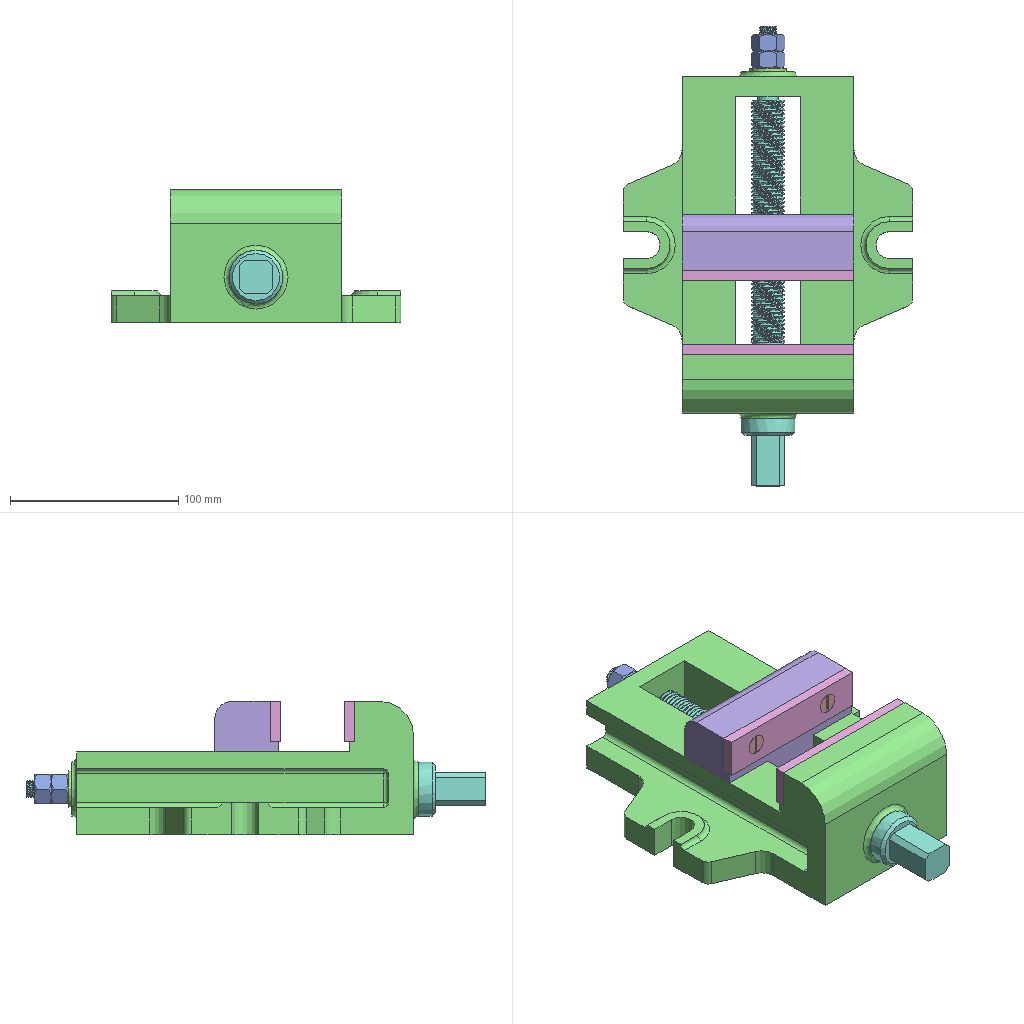Assembly | NX | 8 different items | 15 placed | box 172 x 273 x 79 mm
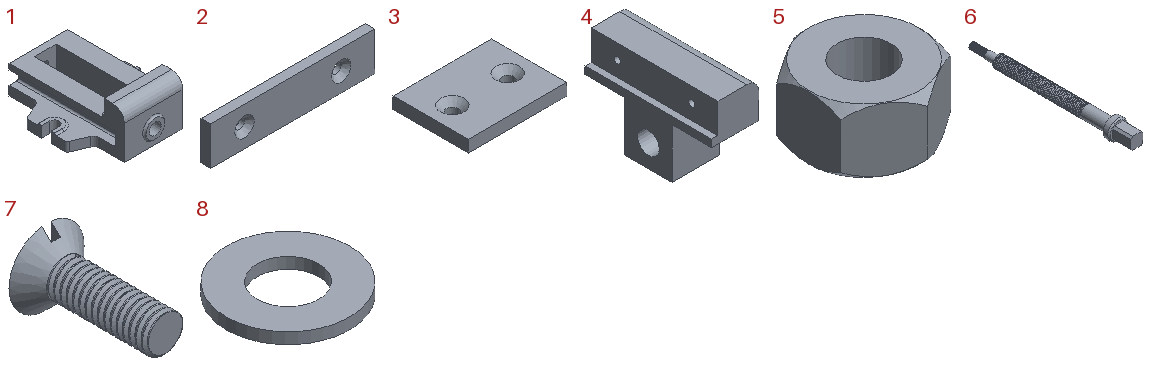Parts list (item | quantity | size | volume | features):
1 | x1 | 172 x 206 x 79 mm | 739526 mm3 | features EXTRUDE 13, BLEND 11, DATUM_CSYS 10, SKETCH 9, EXTRACT_STRING 8, Instance Feature 2, Mirror Feature 2, SIMPLE HOLE 2, SYMBOLIC_THREAD 2, HOLE PACKAGE 1
2 | x2 | 102 x 6 x 24 mm | 14123 mm3 | features DATUM_CSYS 3, CSUNK_HOLE 2, SKETCH 2, EXTRUDE 1, HOLE PACKAGE 1
3 | x1 | 50 x 38 x 6 mm | 10835 mm3 | features DATUM_CSYS 3, CSUNK_HOLE 2, SKETCH 2, EXTRUDE 1, HOLE PACKAGE 1
4 | x1 | 38 x 102 x 70 mm | 149489 mm3 | features DATUM_CSYS 5, SIMPLE HOLE 5, SYMBOLIC_THREAD 5, SKETCH 4, HOLE PACKAGE 3, EXTRUDE 2
5 | x2 | 17.321 x 20 x 10 mm | 2008 mm3 | features DATUM_CSYS 4, SKETCH 3, EXTRACT_STRING 2, SWP104 2, DATUM_PLANE 1, EXTRUDE 1, HOLE PACKAGE 1, Instance Feature 1, Mirror Feature 1, SIMPLE HOLE 1, SYMBOLIC_THREAD 1
6 | x1 | 32 x 273 x 32 mm | 74407 mm3 | features EXTRUDE 8, DATUM_CSYS 7, SKETCH 6, CHAMFER 2, THREADS 2
7 | x6 | 12 x 19 x 11.906 mm | 533.089 mm3 | features DATUM_CSYS 4, SKETCH 3, EXTRUDE 2, SWP104 1, THREADS 1
8 | x1 | 22 x 22 x 2 mm | 570.199 mm3 | features DATUM_CSYS 2, EXTRUDE 1, SKETCH 1
Mates (type | each side: item.copy, entity, surface, feature):
Parallel | 1.1 face plane Extrude(5) | 4.1 face plane Extrude(2)
Parallel | 4.1 face plane Extrude(2) | 1.1 face plane Extrude(2)
Touch | 4.1 face plane Extrude(2) | 1.1 face plane Extrude(5)
Distance | 4.1 face plane Extrude(3) | 1.1 face plane Extrude(2)
Touch | 4.1 face plane Extrude(3) | 1.1 face plane Extrude(2)
Fix | 1.1 component
Concentric | 3.1 edge | 4.1 edge
Concentric | 4.1 edge | 3.1 edge
Concentric | 4.1 edge | 2.1 edge | 2 times
Concentric | 1.1 edge | 6.1 edge
Parallel | 1.1 face plane Extrude(2) | 6.1 face plane Extrude(8)
Concentric | 2.1 edge | 1.1 edge
Concentric | 1.1 edge | 2.1 edge
Concentric | 8.1 edge | 1.1 edge
Touch | 5.1 face cylinder M10 x 1.5 Threaded Hole(7) | 6.1 face cylinder Threads(18) | 2 times
Touch | 8.1 face plane Extrude(1) | 5.1 face plane Extrude(2)
Parallel | 1.1 face plane Extrude(2) | 5.1 face plane Extrude(2)
Touch | 5.1 face plane Extrude(2) | 5.1 face plane Extrude(2)
Parallel | 5.1 face plane Extrude(2) | 5.1 face plane Extrude(2)
Touch | 2.1 face cone Ø6 Countersunk Hole(2) | 7.1 face cylinder Threads(10)
Touch | 7.1 face cone Revolve(4) | 2.1 face cone Ø6 Countersunk Hole(2) | 2 times
Perpendicular | 7.1 face plane Extrude(6) | 1.1 face plane Extrude(2)
Touch | 7.1 face cylinder Threads(10) | 2.1 face cone Ø6 Countersunk Hole(2)
Perpendicular | 1.1 face plane Extrude(2) | 7.1 face plane Extrude(6)
Touch | 7.1 face cylinder Extrude(2) | 4.1 face cylinder M6 x 1.0 Threaded Hole(6)
Touch | 2.1 face cone Ø6 Countersunk Hole(2) | 7.1 face cone Revolve(4) | 2 times
Perpendicular | 7.1 face plane Extrude(6) | 4.1 arc
Perpendicular | 4.1 face plane Extrude(3) | 7.1 face plane Extrude(6) | 2 times
Touch | 7.1 face cylinder Extrude(2) | 2.1 face cone Ø6 Countersunk Hole(2)
Touch | 7.1 face cylinder Threads(10) | 4.1 face cylinder M6 x 1.0 Threaded Hole(5)
Touch | 3.1 face cone Ø6 Countersunk Hole(3) | 7.1 face cone Revolve(4) | 2 times
Parallel | 3.1 face plane Extrude(2) | 7.1 face plane Extrude(6)
Touch | 7.1 face cylinder Threads(10) | 3.1 face cylinder Ø6 Countersunk Hole(3)
Parallel | 7.1 face plane Extrude(6) | 7.1 face plane Extrude(6)